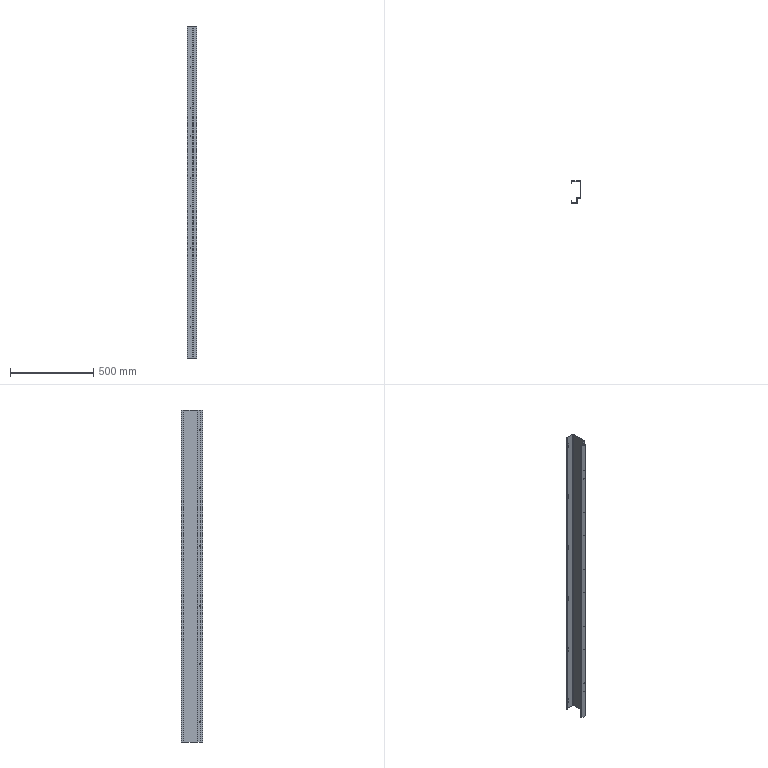Part | 1 solid | 118 faces | box 58 x 130 x 2000 mm | volume 624332 mm3 | cylinder 64 | plane 54 | commonest cylinder face diameters 5 x20 9 x18 4.6 x14 2 x6 4.4 x6